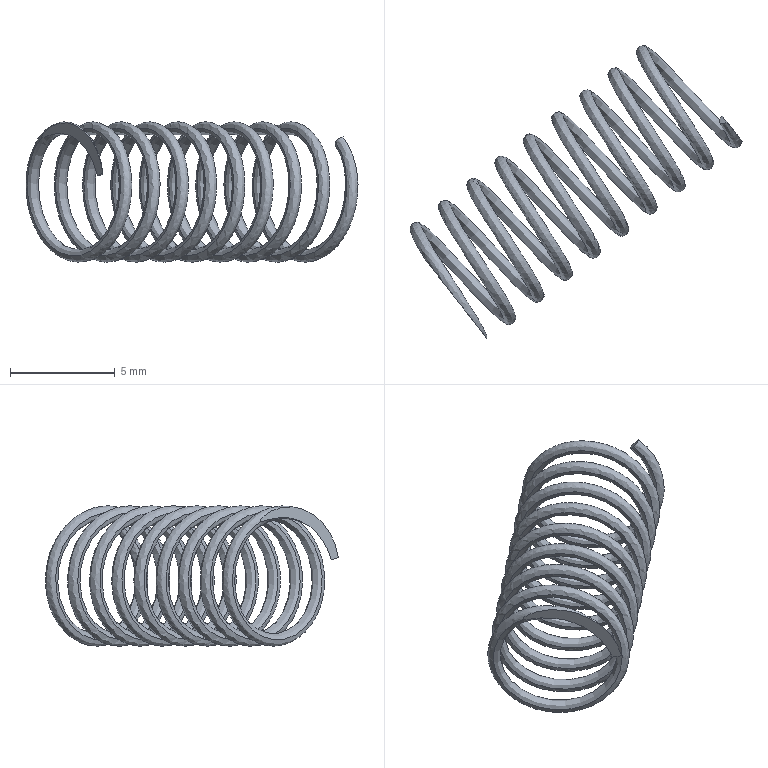Part | SolidWorks | features BaseBody 1 | 1 solid | 6 faces | box 15.796 x 14.132 x 6.7 mm | volume 48.811 mm3 | plane 4 | spline 2